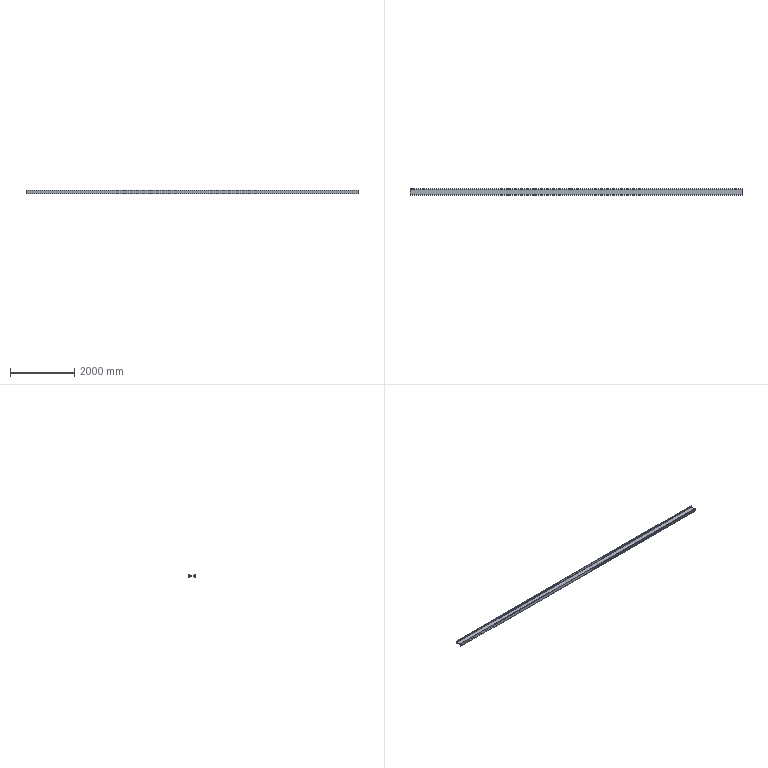Part | STEP file | E3-导轨工字钢1_Default<As Machined> | 1 solid | 62 faces | box 10320 x 200 x 102 mm | volume 40766412 mm3 | cylinder 48 | plane 14 | commonest cylinder face diameters 18 x44 9 x4